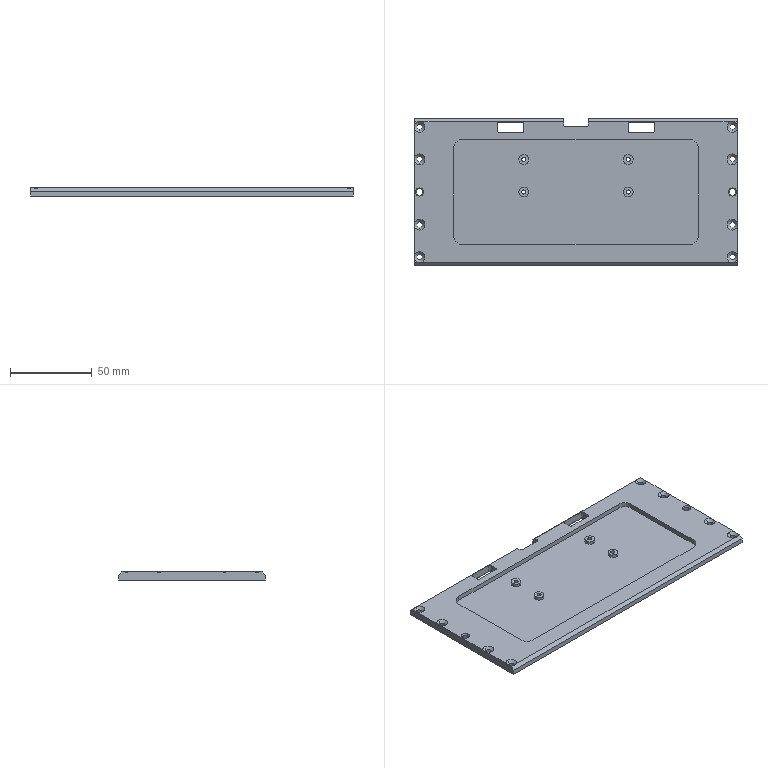NC program | NX | posted with a generic post | part box 198 x 90 x 5 mm
Whole program:
N10 G17 G21 G94 G90
(PLANAR_MILL_COPY_COPY_COPY_COPY_COPY_COPY_2 , TOOL : D6A45)
N12 T01 M6
N14 G54
N16 G17 G0 G90 X96.689 Y-40.412 S9500 M3
N18 G43 Z30. H1
N20 Z0.5
N22 G94 G1 X96.8 Y-40.221 Z0.441 F1250.
N24 Y-39.779 Z0.322
N26 X96.587 Y-39.413 Z0.209
N28 X96.221 Y-39.2 Z0.095
N30 X95.779 Z-0.023
N32 X95.413 Y-39.413 Z-0.137
N34 X95.2 Y-39.779 Z-0.25
N36 Y-40.221 Z-0.369
N38 X95.413 Y-40.587 Z-0.482
N40 X95.779 Y-40.8 Z-0.595
N42 X96.221 Z-0.714
N44 X96.587 Y-40.587 Z-0.827
N46 X96.8 Y-40.221 Z-0.941
N48 Y-40. Z-1.
N50 G3 X96. Y-39.2 R0.8
N52 X96.8 Y-40. R-0.8
N54 X96.55 Y-39.567 R0.5
N56 G1 Z0.5
N58 G0 Z30.
N60 X96.689 Y-20.412
N62 Z0.5
N64 G1 X96.8 Y-20.221 Z0.441
N66 Y-19.779 Z0.322
N68 X96.587 Y-19.413 Z0.209
N70 X96.221 Y-19.2 Z0.095
N72 X95.779 Z-0.023
N74 X95.413 Y-19.413 Z-0.137
N76 X95.2 Y-19.779 Z-0.25
N78 Y-20.221 Z-0.369
N80 X95.413 Y-20.587 Z-0.482
N82 X95.779 Y-20.8 Z-0.595
N84 X96.221 Z-0.714
N86 X96.587 Y-20.587 Z-0.827
N88 X96.8 Y-20.221 Z-0.941
N90 Y-20. Z-1.
N92 G3 X96. Y-19.2 R0.8
N94 X96.8 Y-20. R-0.8
N96 X96.55 Y-19.567 R0.5
N98 G1 Z0.5
N100 G0 Z30.
N102 X96.325 Y1.063
N104 Z0.5
N106 G1 X96.259 Y1.1 Z0.48
N108 X96. Z0.41
N110 X95.741 Z0.341
N112 X95.201 Y0.799 Z0.175
N114 X94.9 Y0.259 Z0.009
N116 Y-0.259 Z-0.129
N118 X95.201 Y-0.799 Z-0.295
N120 X95.741 Y-1.1 Z-0.461
N122 X96.259 Z-0.599
N124 X96.799 Y-0.799 Z-0.765
N126 X97.1 Y-0.259 Z-0.931
N128 Y0. Z-1.
N130 G3 X96. Y1.1 R1.1
N132 X97.1 Y0. R-1.1
N134 X96.6 Y0.866 R1.
N136 G1 Z0.5
N138 G0 Z30.
N140 X96.689 Y19.588
N142 Z0.5
N144 G1 X96.8 Y19.779 Z0.441
N146 Y20.221 Z0.322
N148 X96.587 Y20.587 Z0.209
N150 X96.221 Y20.8 Z0.095
N152 X95.779 Z-0.023
N154 X95.413 Y20.587 Z-0.137
N156 X95.2 Y20.221 Z-0.25
N158 Y19.779 Z-0.369
N160 X95.413 Y19.413 Z-0.482
N162 X95.779 Y19.2 Z-0.595
N164 X96.221 Z-0.714
N166 X96.587 Y19.413 Z-0.827
N168 X96.8 Y19.779 Z-0.941
N170 Y20. Z-1.
N172 G3 X96. Y20.8 R0.8
N174 X96.8 Y20. R-0.8
N176 X96.55 Y20.433 R0.5
N178 G1 Z0.5
N180 G0 Z30.
N182 X96.689 Y39.588
N184 Z0.5
N186 G1 X96.8 Y39.779 Z0.441
N188 Y40.221 Z0.322
N190 X96.587 Y40.587 Z0.209
N192 X96.221 Y40.8 Z0.095
N194 X95.779 Z-0.023
N196 X95.413 Y40.587 Z-0.137
N198 X95.2 Y40.221 Z-0.25
N200 Y39.779 Z-0.369
N202 X95.413 Y39.413 Z-0.482
N204 X95.779 Y39.2 Z-0.595
N206 X96.221 Z-0.714
N208 X96.587 Y39.413 Z-0.827
N210 X96.8 Y39.779 Z-0.941
N212 Y40. Z-1.
N214 G3 X96. Y40.8 R0.8
N216 X96.8 Y40. R-0.8
N218 X96.55 Y40.433 R0.5
N220 G1 Z0.5
N222 G0 Z30.
N224 X41.27 Y40.6
N226 Z0.5
N228 G1 Z-1.
N230 X40.866 Y41.3
N232 G3 X40. Y41.8 R1.
N234 G1 X32.9
N236 X32.835 Y41.813
N238 X32.787 Y41.765
N240 X32.8 Y41.7
N242 Y37.5
N244 X32.787 Y37.435
N246 X32.835 Y37.387
N248 X32.9 Y37.4
N250 X47.1
N252 X47.165 Y37.387
N254 X47.213 Y37.435
N256 X47.2 Y37.5
N258 Y41.7
N260 X47.213 Y41.765
N262 X47.165 Y41.813
N264 X47.1 Y41.8
N266 X40.
N268 G3 X39.134 Y41.3 R1.
N270 G1 X38.73 Y40.6
N272 Z0.5
N274 G0 Z30.
N276 X32.198 Y19.7
N278 Z0.5
N280 G1 X32.35 Y19.852 Z0.442
N282 Y20.148 Z0.363
N284 X32.148 Y20.35 Z0.287
N286 X31.852 Z0.207
N288 X31.65 Y20.148 Z0.131
N290 Y19.852 Z0.051
N292 X31.852 Y19.65 Z-0.025
N294 X32.148 Z-0.105
N296 X32.35 Y19.852 Z-0.181
N298 Y20.148 Z-0.26
N300 X32.148 Y20.35 Z-0.337
N302 X31.852 Z-0.416
N304 X31.65 Y20.148 Z-0.493
N306 Y19.852 Z-0.572
N308 X31.852 Y19.65 Z-0.649
N310 X32.148 Z-0.728
N312 X32.35 Y19.852 Z-0.804
N314 Y20.148 Z-0.884
N316 X32.148 Y20.35 Z-0.96
N318 X32. Z-1.
N320 G3 X31.65 Y20. R0.35
N322 X32. Y20.35 R-0.35
N324 X32.217 Y19.9 R0.5
N326 G1 Z0.5
N328 G0 Z30.
N330 X31.802 Y0.3
N332 Z0.5
N334 G1 X31.65 Y0.148 Z0.442
N336 Y-0.148 Z0.363
N338 X31.852 Y-0.35 Z0.287
N340 X32.148 Z0.207
N342 X32.35 Y-0.148 Z0.131
N344 Y0.148 Z0.051
N346 X32.148 Y0.35 Z-0.025
N348 X31.852 Z-0.105
N350 X31.65 Y0.148 Z-0.181
N352 Y-0.148 Z-0.26
N354 X31.852 Y-0.35 Z-0.337
N356 X32.148 Z-0.416
N358 X32.35 Y-0.148 Z-0.493
N360 Y0.148 Z-0.572
N362 X32.148 Y0.35 Z-0.649
N364 X31.852 Z-0.728
N366 X31.65 Y0.148 Z-0.804
N368 Y-0.148 Z-0.884
N370 X31.852 Y-0.35 Z-0.96
N372 X32. Z-1.
N374 G3 X32.35 Y0. R0.35
N376 X32. Y-0.35 R-0.35
N378 X31.783 Y0.1 R0.5
N380 G1 Z0.5
N382 G0 Z30.
N384 X1.27 Y-47.1
N386 Z0.5
N388 G1 Z-1.
N390 X0.866 Y-46.4
N392 G3 X0. Y-45.9 R1.
N394 G1 X-98.9
N396 G2 X-99.9 Y-44.9 R1.
N398 G1 Y44.9
N400 G2 X-98.9 Y45.9 R1.
N402 G1 X-7.6
N404 G2 X-6.6 Y44.9 R1.
N406 G1 Y41.
N408 X-6.613 Y40.935
N410 X-6.565 Y40.887
N412 X-6.5 Y40.9
N414 X6.5
N416 X6.565 Y40.887
N418 X6.613 Y40.935
N420 X6.6 Y41.
N422 Y44.9
N424 G2 X7.6 Y45.9 R1.
N426 G1 X98.9
N428 G2 X99.9 Y44.9 R1.
N430 G1 Y-44.9
N432 G2 X98.9 Y-45.9 R1.
N434 G1 X0.
N436 G3 X-0.866 Y-46.4 R1.
N438 G1 X-1.27 Y-47.1
N440 Z0.5
N442 G0 Z30.
N444 X-32.198 Y0.3
N446 Z0.5
N448 G1 X-32.35 Y0.148 Z0.442
N450 Y-0.148 Z0.363
N452 X-32.148 Y-0.35 Z0.287
N454 X-31.852 Z0.207
N456 X-31.65 Y-0.148 Z0.131
N458 Y0.148 Z0.051
N460 X-31.852 Y0.35 Z-0.025
N462 X-32.148 Z-0.105
N464 X-32.35 Y0.148 Z-0.181
N466 Y-0.148 Z-0.26
N468 X-32.148 Y-0.35 Z-0.337
N470 X-31.852 Z-0.416
N472 X-31.65 Y-0.148 Z-0.493
N474 Y0.148 Z-0.572
N476 X-31.852 Y0.35 Z-0.649
N478 X-32.148 Z-0.728
N480 X-32.35 Y0.148 Z-0.804
N482 Y-0.148 Z-0.884
N484 X-32.148 Y-0.35 Z-0.96
N486 X-32. Z-1.
N488 G3 X-31.65 Y0. R0.35
N490 X-32. Y-0.35 R-0.35
N492 X-32.217 Y0.1 R0.5
N494 G1 Z0.5
N496 G0 Z30.
N498 X-31.802 Y19.7
N500 Z0.5
N502 G1 X-31.65 Y19.852 Z0.442
N504 Y20.148 Z0.363
N506 X-31.852 Y20.35 Z0.287
N508 X-32.148 Z0.207
N510 X-32.35 Y20.148 Z0.131
N512 Y19.852 Z0.051
N514 X-32.148 Y19.65 Z-0.025
N516 X-31.852 Z-0.105
N518 X-31.65 Y19.852 Z-0.181
N520 Y20.148 Z-0.26
N522 X-31.852 Y20.35 Z-0.337
N524 X-32.148 Z-0.416
N526 X-32.35 Y20.148 Z-0.493
N528 Y19.852 Z-0.572
N530 X-32.148 Y19.65 Z-0.649
N532 X-31.852 Z-0.728
N534 X-31.65 Y19.852 Z-0.804
N536 Y20.148 Z-0.884
N538 X-31.852 Y20.35 Z-0.96
N540 X-32. Z-1.
N542 G3 X-32.35 Y20. R0.35
N544 X-32. Y20.35 R-0.35
N546 X-31.783 Y19.9 R0.5
N548 G1 Z0.5
N550 G0 Z30.
N552 X-38.73 Y40.6
N554 Z0.5
N556 G1 Z-1.
N558 X-39.134 Y41.3
N560 G3 X-40. Y41.8 R1.
N562 G1 X-47.1
N564 X-47.165 Y41.813
N566 X-47.213 Y41.765
N568 X-47.2 Y41.7
N570 Y37.5
N572 X-47.213 Y37.435
N574 X-47.165 Y37.387
N576 X-47.1 Y37.4
N578 X-32.9
N580 X-32.835 Y37.387
N582 X-32.787 Y37.435
N584 X-32.8 Y37.5
N586 Y41.7
N588 X-32.787 Y41.765
N590 X-32.835 Y41.813
N592 X-32.9 Y41.8
N594 X-40.
N596 G3 X-40.866 Y41.3 R1.
N598 G1 X-41.27 Y40.6
N600 Z0.5
N602 G0 Z30.
N604 X-96.689 Y40.412
N606 Z0.5
N608 G1 X-96.8 Y40.221 Z0.441
N610 Y39.779 Z0.322
N612 X-96.587 Y39.413 Z0.209
N614 X-96.221 Y39.2 Z0.095
N616 X-95.779 Z-0.023
N618 X-95.413 Y39.413 Z-0.137
N620 X-95.2 Y39.779 Z-0.25
N622 Y40.221 Z-0.369
N624 X-95.413 Y40.587 Z-0.482
N626 X-95.779 Y40.8 Z-0.595
N628 X-96.221 Z-0.714
N630 X-96.587 Y40.587 Z-0.827
N632 X-96.8 Y40.221 Z-0.941
N634 Y40. Z-1.
N636 G3 X-96. Y39.2 R0.8
N638 X-96.8 Y40. R-0.8
N640 X-96.55 Y39.567 R0.5
N642 G1 Z0.5
N644 G0 Z30.
N646 X-96.689 Y20.412
N648 Z0.5
N650 G1 X-96.8 Y20.221 Z0.441
N652 Y19.779 Z0.322
N654 X-96.587 Y19.413 Z0.209
N656 X-96.221 Y19.2 Z0.095
N658 X-95.779 Z-0.023
N660 X-95.413 Y19.413 Z-0.137
N662 X-95.2 Y19.779 Z-0.25
N664 Y20.221 Z-0.369
N666 X-95.413 Y20.587 Z-0.482
N668 X-95.779 Y20.8 Z-0.595
N670 X-96.221 Z-0.714
N672 X-96.587 Y20.587 Z-0.827
N674 X-96.8 Y20.221 Z-0.941
N676 Y20. Z-1.
N678 G3 X-96. Y19.2 R0.8
N680 X-96.8 Y20. R-0.8
N682 X-96.55 Y19.567 R0.5
N684 G1 Z0.5
N686 G0 Z30.
N688 X-96.325 Y-1.063
N690 Z0.5
N692 G1 X-96.259 Y-1.1 Z0.48
N694 X-96. Z0.41
N696 X-95.741 Z0.341
N698 X-95.201 Y-0.799 Z0.175
N700 X-94.9 Y-0.259 Z0.009
N702 Y0.259 Z-0.129
N704 X-95.201 Y0.799 Z-0.295
N706 X-95.741 Y1.1 Z-0.461
N708 X-96.259 Z-0.599
N710 X-96.799 Y0.799 Z-0.765
N712 X-97.1 Y0.259 Z-0.931
N714 Y0. Z-1.
N716 G3 X-96. Y-1.1 R1.1
N718 X-97.1 Y0. R-1.1
N720 X-96.6 Y-0.866 R1.
N722 G1 Z0.5
N724 G0 Z30.
N726 X-96.689 Y-19.588
N728 Z0.5
N730 G1 X-96.8 Y-19.779 Z0.441
N732 Y-20.221 Z0.322
N734 X-96.587 Y-20.587 Z0.209
N736 X-96.221 Y-20.8 Z0.095
N738 X-95.779 Z-0.023
N740 X-95.413 Y-20.587 Z-0.137
N742 X-95.2 Y-20.221 Z-0.25
N744 Y-19.779 Z-0.369
N746 X-95.413 Y-19.413 Z-0.482
N748 X-95.779 Y-19.2 Z-0.595
N750 X-96.221 Z-0.714
N752 X-96.587 Y-19.413 Z-0.827
N754 X-96.8 Y-19.779 Z-0.941
N756 Y-20. Z-1.
N758 G3 X-96. Y-20.8 R0.8
N760 X-96.8 Y-20. R-0.8
N762 X-96.55 Y-20.433 R0.5
N764 G1 Z0.5
N766 G0 Z30.
N768 X-96.689 Y-39.588
N770 Z0.5
N772 G1 X-96.8 Y-39.779 Z0.441
N774 Y-40.221 Z0.322
N776 X-96.587 Y-40.587 Z0.209
N778 X-96.221 Y-40.8 Z0.095
N780 X-95.779 Z-0.023
N782 X-95.413 Y-40.587 Z-0.137
N784 X-95.2 Y-40.221 Z-0.25
N786 Y-39.779 Z-0.369
N788 X-95.413 Y-39.413 Z-0.482
N790 X-95.779 Y-39.2 Z-0.595
N792 X-96.221 Z-0.714
N794 X-96.587 Y-39.413 Z-0.827
N796 X-96.8 Y-39.779 Z-0.941
N798 Y-40. Z-1.
N800 G3 X-96. Y-40.8 R0.8
N802 X-96.8 Y-40. R-0.8
N804 X-96.55 Y-40.433 R0.5
N806 G1 Z0.5
N808 G0 Z30.
(PLANAR_MILL_COPY_COPY_COPY_COPY_COPY_COPY_1_1 , TOOL : D6A45)
N810 X-40.866 Y38.
N812 Z0.
N814 G1 Z-1.5
N816 G3 X-40. Y37.5 R1.
N818 G1 X-32.9
N820 Y41.7
N822 X-47.1
N824 Y37.5
N826 X-40.
N828 G3 X-39.134 Y38. R1.
N830 G1 Z0.
N832 G0 Z30.
N834 X40.866 Y41.2
N836 Z0.
N838 G1 Z-1.5
N840 G3 X40. Y41.7 R1.
N842 G1 X32.9
N844 Y37.5
N846 X47.1
N848 Y41.7
N850 X40.
N852 G3 X39.134 Y41.2 R1.
N854 G1 Z0.
N856 G0 Z30.
N858 M5
N860 M2